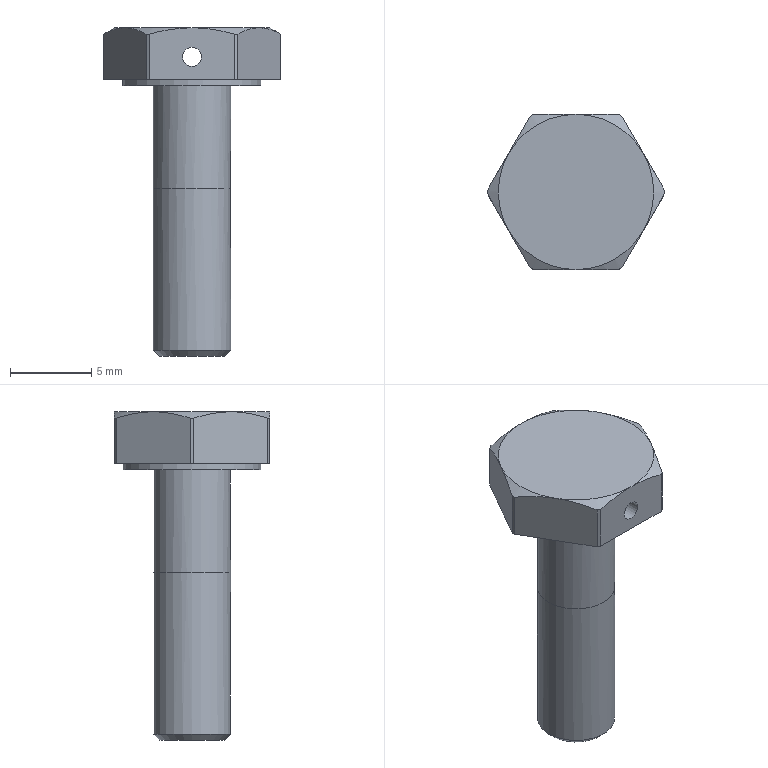Part | NX | features solid 2 | 1 solid | 27 faces | box 10.922 x 9.576 x 20.25 mm | volume 559.779 mm3 | cylinder 10 | plane 10 | cone 7 | commonest cylinder face diameters 10.922 x6 4.763 x2 1.168 x1 8.509 x1
STEP:
#1=CARTESIAN_POINT('',(-2.381,0.,-3.581));
#2=VERTEX_POINT('',#1);
#3=CARTESIAN_POINT('',(0.,0.,-3.581));
#4=DIRECTION('',(0.,0.,-1.));
#5=DIRECTION('',(-1.,0.,0.));
#6=AXIS2_PLACEMENT_3D('',#3,#4,#5);
#7=CIRCLE('',#6,2.381);
#8=EDGE_CURVE('',#2,#2,#7,.T.);
#9=ORIENTED_EDGE('',*,*,#8,.T.);
#10=EDGE_LOOP('',(#9));
#11=FACE_BOUND('',#10,.T.);
#12=CARTESIAN_POINT('',(-2.381,0.,-9.931));
#13=VERTEX_POINT('',#12);
#14=CARTESIAN_POINT('',(-1.866,1.866,-9.931));
#15=CARTESIAN_POINT('',(-2.639,0.,-9.931));
#16=CARTESIAN_POINT('',(-1.866,-1.866,-9.931));
#17=CARTESIAN_POINT('',(0.,-2.639,-9.931));
#18=CARTESIAN_POINT('',(1.866,-1.866,-9.931));
#19=CARTESIAN_POINT('',(2.639,0.,-9.931));
#20=CARTESIAN_POINT('',(1.866,1.866,-9.931));
#21=CARTESIAN_POINT('',(0.,2.639,-9.931));
#22=CARTESIAN_POINT('',(-1.866,1.866,-9.931));
#23=CARTESIAN_POINT('',(-2.639,0.,-9.931));
#24=CARTESIAN_POINT('',(-1.866,-1.866,-9.931));
#25=B_SPLINE_CURVE_WITH_KNOTS('',3,(#14,#15,#16,#17,#18,#19,#20,#21,#22,#23,#24),.UNSPECIFIED.,.T.,.F.,(1,1,1,1,1,1,1,1,1,1,1,1,1,1,1),(-0.375,-0.25,-0.125,0.,0.125,0.25,0.375,0.5,0.625,0.75,0.875,1.,1.125,1.25,1.375),.UNSPECIFIED.);
#26=EDGE_CURVE('',#13,#13,#25,.T.);
#27=ORIENTED_EDGE('',*,*,#26,.T.);
#28=EDGE_LOOP('',(#27));
#29=FACE_BOUND('',#28,.T.);
#30=CARTESIAN_POINT('',(0.,0.,0.));
#31=DIRECTION('',(0.,0.,-1.));
#32=DIRECTION('',(-1.,0.,0.));
#33=AXIS2_PLACEMENT_3D('',#30,#31,#32);
#34=CYLINDRICAL_SURFACE('',#33,2.381);
#35=ADVANCED_FACE('',(#11,#29),#34,.T.);
#36=CARTESIAN_POINT('',(2.627,4.788,-3.175));
#37=VERTEX_POINT('',#36);
#38=CARTESIAN_POINT('',(2.833,4.669,-3.175));
#39=VERTEX_POINT('',#38);
#40=CARTESIAN_POINT('',(0.,0.,-3.175));
#41=DIRECTION('',(0.,0.,-1.));
#42=DIRECTION('',(-1.,0.,0.));
#43=AXIS2_PLACEMENT_3D('',#40,#41,#42);
#44=CIRCLE('',#43,5.461);
#45=EDGE_CURVE('',#37,#39,#44,.T.);
#46=ORIENTED_EDGE('',*,*,#45,.F.);
#47=CARTESIAN_POINT('',(2.627,4.788,-0.3886));
#48=VERTEX_POINT('',#47);
#49=CARTESIAN_POINT('',(2.627,4.788,0.));
#50=DIRECTION('',(0.,0.,-1.));
#51=VECTOR('',#50,1000.);
#52=LINE('',#49,#51);
#53=EDGE_CURVE('',#37,#48,#52,.F.);
#54=ORIENTED_EDGE('',*,*,#53,.T.);
#55=CARTESIAN_POINT('',(2.833,4.669,-0.3886));
#56=VERTEX_POINT('',#55);
#57=CARTESIAN_POINT('',(0.,0.,-0.3886));
#58=DIRECTION('',(0.,0.,-1.));
#59=DIRECTION('',(-1.,0.,0.));
#60=AXIS2_PLACEMENT_3D('',#57,#58,#59);
#61=CIRCLE('',#60,5.461);
#62=EDGE_CURVE('',#48,#56,#61,.T.);
#63=ORIENTED_EDGE('',*,*,#62,.T.);
#64=CARTESIAN_POINT('',(2.833,4.669,0.));
#65=DIRECTION('',(0.,0.,-1.));
#66=VECTOR('',#65,1000.);
#67=LINE('',#64,#66);
#68=EDGE_CURVE('',#56,#39,#67,.T.);
#69=ORIENTED_EDGE('',*,*,#68,.T.);
#70=EDGE_LOOP('',(#46,#54,#63,#69));
#71=FACE_BOUND('',#70,.T.);
#72=CARTESIAN_POINT('',(0.,0.,0.));
#73=DIRECTION('',(0.,0.,-1.));
#74=DIRECTION('',(-1.,0.,0.));
#75=AXIS2_PLACEMENT_3D('',#72,#73,#74);
#76=CYLINDRICAL_SURFACE('',#75,5.461);
#77=ADVANCED_FACE('',(#71),#76,.T.);
#78=CARTESIAN_POINT('',(-2.833,4.669,-0.3886));
#79=VERTEX_POINT('',#78);
#80=CARTESIAN_POINT('',(-2.627,4.788,-0.3886));
#81=VERTEX_POINT('',#80);
#82=CARTESIAN_POINT('',(0.,0.,-0.3886));
#83=DIRECTION('',(0.,0.,-1.));
#84=DIRECTION('',(-1.,0.,0.));
#85=AXIS2_PLACEMENT_3D('',#82,#83,#84);
#86=CIRCLE('',#85,5.461);
#87=EDGE_CURVE('',#79,#81,#86,.T.);
#88=ORIENTED_EDGE('',*,*,#87,.T.);
#89=CARTESIAN_POINT('',(-2.627,4.788,-3.175));
#90=VERTEX_POINT('',#89);
#91=CARTESIAN_POINT('',(-2.627,4.788,0.));
#92=DIRECTION('',(0.,0.,-1.));
#93=VECTOR('',#92,1000.);
#94=LINE('',#91,#93);
#95=EDGE_CURVE('',#81,#90,#94,.T.);
#96=ORIENTED_EDGE('',*,*,#95,.T.);
#97=CARTESIAN_POINT('',(-2.833,4.669,-3.175));
#98=VERTEX_POINT('',#97);
#99=CARTESIAN_POINT('',(0.,0.,-3.175));
#100=DIRECTION('',(0.,0.,-1.));
#101=DIRECTION('',(-1.,0.,0.));
#102=AXIS2_PLACEMENT_3D('',#99,#100,#101);
#103=CIRCLE('',#102,5.461);
#104=EDGE_CURVE('',#98,#90,#103,.T.);
#105=ORIENTED_EDGE('',*,*,#104,.F.);
#106=CARTESIAN_POINT('',(-2.833,4.669,0.));
#107=DIRECTION('',(0.,0.,-1.));
#108=VECTOR('',#107,1000.);
#109=LINE('',#106,#108);
#110=EDGE_CURVE('',#98,#79,#109,.F.);
#111=ORIENTED_EDGE('',*,*,#110,.T.);
#112=EDGE_LOOP('',(#88,#96,#105,#111));
#113=FACE_BOUND('',#112,.T.);
#114=CARTESIAN_POINT('',(0.,0.,0.));
#115=DIRECTION('',(0.,0.,-1.));
#116=DIRECTION('',(-1.,0.,0.));
#117=AXIS2_PLACEMENT_3D('',#114,#115,#116);
#118=CYLINDRICAL_SURFACE('',#117,5.461);
#119=ADVANCED_FACE('',(#113),#118,.T.);
#120=CARTESIAN_POINT('',(-5.46,-0.1193,-0.3886));
#121=VERTEX_POINT('',#120);
#122=CARTESIAN_POINT('',(-5.46,0.1193,-0.3886));
#123=VERTEX_POINT('',#122);
#124=CARTESIAN_POINT('',(0.,0.,-0.3886));
#125=DIRECTION('',(0.,0.,-1.));
#126=DIRECTION('',(-1.,0.,0.));
#127=AXIS2_PLACEMENT_3D('',#124,#125,#126);
#128=CIRCLE('',#127,5.461);
#129=EDGE_CURVE('',#121,#123,#128,.T.);
#130=ORIENTED_EDGE('',*,*,#129,.T.);
#131=CARTESIAN_POINT('',(-5.46,0.1193,-3.175));
#132=VERTEX_POINT('',#131);
#133=CARTESIAN_POINT('',(-5.46,0.1193,0.));
#134=DIRECTION('',(0.,0.,-1.));
#135=VECTOR('',#134,1000.);
#136=LINE('',#133,#135);
#137=EDGE_CURVE('',#123,#132,#136,.T.);
#138=ORIENTED_EDGE('',*,*,#137,.T.);
#139=CARTESIAN_POINT('',(-5.46,-0.1193,-3.175));
#140=VERTEX_POINT('',#139);
#141=CARTESIAN_POINT('',(0.,0.,-3.175));
#142=DIRECTION('',(0.,0.,-1.));
#143=DIRECTION('',(-1.,0.,0.));
#144=AXIS2_PLACEMENT_3D('',#141,#142,#143);
#145=CIRCLE('',#144,5.461);
#146=EDGE_CURVE('',#140,#132,#145,.T.);
#147=ORIENTED_EDGE('',*,*,#146,.F.);
#148=CARTESIAN_POINT('',(-5.46,-0.1193,0.));
#149=DIRECTION('',(0.,0.,-1.));
#150=VECTOR('',#149,1000.);
#151=LINE('',#148,#150);
#152=EDGE_CURVE('',#140,#121,#151,.F.);
#153=ORIENTED_EDGE('',*,*,#152,.T.);
#154=EDGE_LOOP('',(#130,#138,#147,#153));
#155=FACE_BOUND('',#154,.T.);
#156=CARTESIAN_POINT('',(0.,0.,0.));
#157=DIRECTION('',(0.,0.,-1.));
#158=DIRECTION('',(-1.,0.,0.));
#159=AXIS2_PLACEMENT_3D('',#156,#157,#158);
#160=CYLINDRICAL_SURFACE('',#159,5.461);
#161=ADVANCED_FACE('',(#155),#160,.T.);
#162=CARTESIAN_POINT('',(-2.627,-4.788,-0.3886));
#163=VERTEX_POINT('',#162);
#164=CARTESIAN_POINT('',(-2.833,-4.669,-0.3886));
#165=VERTEX_POINT('',#164);
#166=CARTESIAN_POINT('',(0.,0.,-0.3886));
#167=DIRECTION('',(0.,0.,-1.));
#168=DIRECTION('',(-1.,0.,0.));
#169=AXIS2_PLACEMENT_3D('',#166,#167,#168);
#170=CIRCLE('',#169,5.461);
#171=EDGE_CURVE('',#163,#165,#170,.T.);
#172=ORIENTED_EDGE('',*,*,#171,.T.);
#173=CARTESIAN_POINT('',(-2.833,-4.669,-3.175));
#174=VERTEX_POINT('',#173);
#175=CARTESIAN_POINT('',(-2.833,-4.669,0.));
#176=DIRECTION('',(0.,0.,-1.));
#177=VECTOR('',#176,1000.);
#178=LINE('',#175,#177);
#179=EDGE_CURVE('',#165,#174,#178,.T.);
#180=ORIENTED_EDGE('',*,*,#179,.T.);
#181=CARTESIAN_POINT('',(-2.627,-4.788,-3.175));
#182=VERTEX_POINT('',#181);
#183=CARTESIAN_POINT('',(0.,0.,-3.175));
#184=DIRECTION('',(0.,0.,-1.));
#185=DIRECTION('',(-1.,0.,0.));
#186=AXIS2_PLACEMENT_3D('',#183,#184,#185);
#187=CIRCLE('',#186,5.461);
#188=EDGE_CURVE('',#182,#174,#187,.T.);
#189=ORIENTED_EDGE('',*,*,#188,.F.);
#190=CARTESIAN_POINT('',(-2.627,-4.788,0.));
#191=DIRECTION('',(0.,0.,-1.));
#192=VECTOR('',#191,1000.);
#193=LINE('',#190,#192);
#194=EDGE_CURVE('',#182,#163,#193,.F.);
#195=ORIENTED_EDGE('',*,*,#194,.T.);
#196=EDGE_LOOP('',(#172,#180,#189,#195));
#197=FACE_BOUND('',#196,.T.);
#198=CARTESIAN_POINT('',(0.,0.,0.));
#199=DIRECTION('',(0.,0.,-1.));
#200=DIRECTION('',(-1.,0.,0.));
#201=AXIS2_PLACEMENT_3D('',#198,#199,#200);
#202=CYLINDRICAL_SURFACE('',#201,5.461);
#203=ADVANCED_FACE('',(#197),#202,.T.);
#204=CARTESIAN_POINT('',(2.833,-4.669,-0.3886));
#205=VERTEX_POINT('',#204);
#206=CARTESIAN_POINT('',(2.627,-4.788,-0.3886));
#207=VERTEX_POINT('',#206);
#208=CARTESIAN_POINT('',(0.,0.,-0.3886));
#209=DIRECTION('',(0.,0.,-1.));
#210=DIRECTION('',(-1.,0.,0.));
#211=AXIS2_PLACEMENT_3D('',#208,#209,#210);
#212=CIRCLE('',#211,5.461);
#213=EDGE_CURVE('',#205,#207,#212,.T.);
#214=ORIENTED_EDGE('',*,*,#213,.T.);
#215=CARTESIAN_POINT('',(2.627,-4.788,-3.175));
#216=VERTEX_POINT('',#215);
#217=CARTESIAN_POINT('',(2.627,-4.788,0.));
#218=DIRECTION('',(0.,0.,-1.));
#219=VECTOR('',#218,1000.);
#220=LINE('',#217,#219);
#221=EDGE_CURVE('',#207,#216,#220,.T.);
#222=ORIENTED_EDGE('',*,*,#221,.T.);
#223=CARTESIAN_POINT('',(2.833,-4.669,-3.175));
#224=VERTEX_POINT('',#223);
#225=CARTESIAN_POINT('',(0.,0.,-3.175));
#226=DIRECTION('',(0.,0.,-1.));
#227=DIRECTION('',(-1.,0.,0.));
#228=AXIS2_PLACEMENT_3D('',#225,#226,#227);
#229=CIRCLE('',#228,5.461);
#230=EDGE_CURVE('',#224,#216,#229,.T.);
#231=ORIENTED_EDGE('',*,*,#230,.F.);
#232=CARTESIAN_POINT('',(2.833,-4.669,0.));
#233=DIRECTION('',(0.,0.,-1.));
#234=VECTOR('',#233,1000.);
#235=LINE('',#232,#234);
#236=EDGE_CURVE('',#224,#205,#235,.F.);
#237=ORIENTED_EDGE('',*,*,#236,.T.);
#238=EDGE_LOOP('',(#214,#222,#231,#237));
#239=FACE_BOUND('',#238,.T.);
#240=CARTESIAN_POINT('',(0.,0.,0.));
#241=DIRECTION('',(0.,0.,-1.));
#242=DIRECTION('',(-1.,0.,0.));
#243=AXIS2_PLACEMENT_3D('',#240,#241,#242);
#244=CYLINDRICAL_SURFACE('',#243,5.461);
#245=ADVANCED_FACE('',(#239),#244,.T.);
#246=ORIENTED_EDGE('',*,*,#62,.F.);
#247=CARTESIAN_POINT('',(0.,4.788,0.));
#248=VERTEX_POINT('',#247);
#249=CARTESIAN_POINT('',(0.,4.788,0.));
#250=CARTESIAN_POINT('',(0.8868,4.788,0.));
#251=CARTESIAN_POINT('',(1.776,4.788,-0.1525));
#252=CARTESIAN_POINT('',(2.627,4.788,-0.3886));
#253=B_SPLINE_CURVE_WITH_KNOTS('',3,(#249,#250,#251,#252),.UNSPECIFIED.,.F.,.F.,(4,4),(0.007722,0.01038),.UNSPECIFIED.);
#254=EDGE_CURVE('',#48,#248,#253,.F.);
#255=ORIENTED_EDGE('',*,*,#254,.T.);
#256=CARTESIAN_POINT('',(4.146,2.394,0.));
#257=VERTEX_POINT('',#256);
#258=CARTESIAN_POINT('',(0.,0.,0.));
#259=DIRECTION('',(0.,0.,-1.));
#260=DIRECTION('',(-1.,0.,0.));
#261=AXIS2_PLACEMENT_3D('',#258,#259,#260);
#262=CIRCLE('',#261,4.788);
#263=EDGE_CURVE('',#248,#257,#262,.T.);
#264=ORIENTED_EDGE('',*,*,#263,.T.);
#265=CARTESIAN_POINT('',(4.146,2.394,0.));
#266=CARTESIAN_POINT('',(3.703,3.163,0.));
#267=CARTESIAN_POINT('',(3.262,3.925,-0.1503));
#268=CARTESIAN_POINT('',(2.833,4.669,-0.3886));
#269=B_SPLINE_CURVE_WITH_KNOTS('',3,(#265,#266,#267,#268),.UNSPECIFIED.,.F.,.F.,(4,4),(0.002655,0.005296),.UNSPECIFIED.);
#270=EDGE_CURVE('',#257,#56,#269,.T.);
#271=ORIENTED_EDGE('',*,*,#270,.T.);
#272=EDGE_LOOP('',(#246,#255,#264,#271));
#273=FACE_BOUND('',#272,.T.);
#274=CARTESIAN_POINT('',(0.,0.,-0.3886));
#275=DIRECTION('',(0.,0.,-1.));
#276=DIRECTION('',(-1.,0.,0.));
#277=AXIS2_PLACEMENT_3D('',#274,#275,#276);
#278=CONICAL_SURFACE('',#277,5.461,1.047);
#279=ADVANCED_FACE('',(#273),#278,.T.);
#280=CARTESIAN_POINT('',(-4.146,2.394,0.));
#281=VERTEX_POINT('',#280);
#282=CARTESIAN_POINT('',(0.,0.,0.));
#283=DIRECTION('',(0.,0.,-1.));
#284=DIRECTION('',(-1.,0.,0.));
#285=AXIS2_PLACEMENT_3D('',#282,#283,#284);
#286=CIRCLE('',#285,4.788);
#287=EDGE_CURVE('',#281,#248,#286,.T.);
#288=ORIENTED_EDGE('',*,*,#287,.T.);
#289=CARTESIAN_POINT('',(-2.627,4.788,-0.3886));
#290=CARTESIAN_POINT('',(-1.77,4.788,-0.1508));
#291=CARTESIAN_POINT('',(-0.8866,4.788,0.));
#292=CARTESIAN_POINT('',(0.,4.788,0.));
#293=B_SPLINE_CURVE_WITH_KNOTS('',3,(#289,#290,#291,#292),.UNSPECIFIED.,.F.,.F.,(4,4),(0.005068,0.007722),.UNSPECIFIED.);
#294=EDGE_CURVE('',#248,#81,#293,.F.);
#295=ORIENTED_EDGE('',*,*,#294,.T.);
#296=ORIENTED_EDGE('',*,*,#87,.F.);
#297=CARTESIAN_POINT('',(-2.833,4.669,-0.3886));
#298=CARTESIAN_POINT('',(-3.264,3.923,-0.1495));
#299=CARTESIAN_POINT('',(-3.7,3.167,0.));
#300=CARTESIAN_POINT('',(-4.146,2.394,0.));
#301=B_SPLINE_CURVE_WITH_KNOTS('',3,(#297,#298,#299,#300),.UNSPECIFIED.,.F.,.F.,(4,4),(0.00000074,0.002655),.UNSPECIFIED.);
#302=EDGE_CURVE('',#79,#281,#301,.T.);
#303=ORIENTED_EDGE('',*,*,#302,.T.);
#304=EDGE_LOOP('',(#288,#295,#296,#303));
#305=FACE_BOUND('',#304,.T.);
#306=CARTESIAN_POINT('',(0.,0.,-0.3886));
#307=DIRECTION('',(0.,0.,-1.));
#308=DIRECTION('',(-1.,0.,0.));
#309=AXIS2_PLACEMENT_3D('',#306,#307,#308);
#310=CONICAL_SURFACE('',#309,5.461,1.047);
#311=ADVANCED_FACE('',(#305),#310,.T.);
#312=CARTESIAN_POINT('',(-4.146,-2.394,0.));
#313=VERTEX_POINT('',#312);
#314=CARTESIAN_POINT('',(0.,0.,0.));
#315=DIRECTION('',(0.,0.,-1.));
#316=DIRECTION('',(-1.,0.,0.));
#317=AXIS2_PLACEMENT_3D('',#314,#315,#316);
#318=CIRCLE('',#317,4.788);
#319=EDGE_CURVE('',#313,#281,#318,.T.);
#320=ORIENTED_EDGE('',*,*,#319,.T.);
#321=CARTESIAN_POINT('',(-4.146,2.394,0.));
#322=CARTESIAN_POINT('',(-4.59,1.625,0.));
#323=CARTESIAN_POINT('',(-5.031,0.8625,-0.1503));
#324=CARTESIAN_POINT('',(-5.46,0.1193,-0.3886));
#325=B_SPLINE_CURVE_WITH_KNOTS('',3,(#321,#322,#323,#324),.UNSPECIFIED.,.F.,.F.,(4,4),(0.002655,0.005296),.UNSPECIFIED.);
#326=EDGE_CURVE('',#281,#123,#325,.T.);
#327=ORIENTED_EDGE('',*,*,#326,.T.);
#328=ORIENTED_EDGE('',*,*,#129,.F.);
#329=CARTESIAN_POINT('',(-5.46,-0.1193,-0.3886));
#330=CARTESIAN_POINT('',(-5.029,-0.8651,-0.1495));
#331=CARTESIAN_POINT('',(-4.593,-1.621,0.));
#332=CARTESIAN_POINT('',(-4.146,-2.394,0.));
#333=B_SPLINE_CURVE_WITH_KNOTS('',3,(#329,#330,#331,#332),.UNSPECIFIED.,.F.,.F.,(4,4),(0.00000074,0.002655),.UNSPECIFIED.);
#334=EDGE_CURVE('',#121,#313,#333,.T.);
#335=ORIENTED_EDGE('',*,*,#334,.T.);
#336=EDGE_LOOP('',(#320,#327,#328,#335));
#337=FACE_BOUND('',#336,.T.);
#338=CARTESIAN_POINT('',(0.,0.,-0.3886));
#339=DIRECTION('',(0.,0.,-1.));
#340=DIRECTION('',(-1.,0.,0.));
#341=AXIS2_PLACEMENT_3D('',#338,#339,#340);
#342=CONICAL_SURFACE('',#341,5.461,1.047);
#343=ADVANCED_FACE('',(#337),#342,.T.);
#344=CARTESIAN_POINT('',(0.,-4.788,0.));
#345=VERTEX_POINT('',#344);
#346=CARTESIAN_POINT('',(0.,0.,0.));
#347=DIRECTION('',(0.,0.,-1.));
#348=DIRECTION('',(-1.,0.,0.));
#349=AXIS2_PLACEMENT_3D('',#346,#347,#348);
#350=CIRCLE('',#349,4.788);
#351=EDGE_CURVE('',#345,#313,#350,.T.);
#352=ORIENTED_EDGE('',*,*,#351,.T.);
#353=CARTESIAN_POINT('',(-4.146,-2.394,0.));
#354=CARTESIAN_POINT('',(-3.703,-3.163,0.));
#355=CARTESIAN_POINT('',(-3.262,-3.925,-0.1503));
#356=CARTESIAN_POINT('',(-2.833,-4.669,-0.3886));
#357=B_SPLINE_CURVE_WITH_KNOTS('',3,(#353,#354,#355,#356),.UNSPECIFIED.,.F.,.F.,(4,4),(0.002655,0.005296),.UNSPECIFIED.);
#358=EDGE_CURVE('',#313,#165,#357,.T.);
#359=ORIENTED_EDGE('',*,*,#358,.T.);
#360=ORIENTED_EDGE('',*,*,#171,.F.);
#361=CARTESIAN_POINT('',(-2.627,-4.788,-0.3886));
#362=CARTESIAN_POINT('',(-1.77,-4.788,-0.1508));
#363=CARTESIAN_POINT('',(-0.8866,-4.788,0.));
#364=CARTESIAN_POINT('',(0.,-4.788,0.));
#365=B_SPLINE_CURVE_WITH_KNOTS('',3,(#361,#362,#363,#364),.UNSPECIFIED.,.F.,.F.,(4,4),(0.005068,0.007722),.UNSPECIFIED.);
#366=EDGE_CURVE('',#163,#345,#365,.T.);
#367=ORIENTED_EDGE('',*,*,#366,.T.);
#368=EDGE_LOOP('',(#352,#359,#360,#367));
#369=FACE_BOUND('',#368,.T.);
#370=CARTESIAN_POINT('',(0.,0.,-0.3886));
#371=DIRECTION('',(0.,0.,-1.));
#372=DIRECTION('',(-1.,0.,0.));
#373=AXIS2_PLACEMENT_3D('',#370,#371,#372);
#374=CONICAL_SURFACE('',#373,5.461,1.047);
#375=ADVANCED_FACE('',(#369),#374,.T.);
#376=CARTESIAN_POINT('',(4.146,-2.394,0.));
#377=VERTEX_POINT('',#376);
#378=CARTESIAN_POINT('',(0.,0.,0.));
#379=DIRECTION('',(0.,0.,-1.));
#380=DIRECTION('',(-1.,0.,0.));
#381=AXIS2_PLACEMENT_3D('',#378,#379,#380);
#382=CIRCLE('',#381,4.788);
#383=EDGE_CURVE('',#377,#345,#382,.T.);
#384=ORIENTED_EDGE('',*,*,#383,.T.);
#385=CARTESIAN_POINT('',(0.,-4.788,0.));
#386=CARTESIAN_POINT('',(0.8868,-4.788,0.));
#387=CARTESIAN_POINT('',(1.776,-4.788,-0.1525));
#388=CARTESIAN_POINT('',(2.627,-4.788,-0.3886));
#389=B_SPLINE_CURVE_WITH_KNOTS('',3,(#385,#386,#387,#388),.UNSPECIFIED.,.F.,.F.,(4,4),(0.007722,0.01038),.UNSPECIFIED.);
#390=EDGE_CURVE('',#345,#207,#389,.T.);
#391=ORIENTED_EDGE('',*,*,#390,.T.);
#392=ORIENTED_EDGE('',*,*,#213,.F.);
#393=CARTESIAN_POINT('',(2.833,-4.669,-0.3886));
#394=CARTESIAN_POINT('',(3.264,-3.923,-0.1495));
#395=CARTESIAN_POINT('',(3.7,-3.167,0.));
#396=CARTESIAN_POINT('',(4.146,-2.394,0.));
#397=B_SPLINE_CURVE_WITH_KNOTS('',3,(#393,#394,#395,#396),.UNSPECIFIED.,.F.,.F.,(4,4),(0.00000074,0.002655),.UNSPECIFIED.);
#398=EDGE_CURVE('',#205,#377,#397,.T.);
#399=ORIENTED_EDGE('',*,*,#398,.T.);
#400=EDGE_LOOP('',(#384,#391,#392,#399));
#401=FACE_BOUND('',#400,.T.);
#402=CARTESIAN_POINT('',(0.,0.,-0.3886));
#403=DIRECTION('',(0.,0.,-1.));
#404=DIRECTION('',(-1.,0.,0.));
#405=AXIS2_PLACEMENT_3D('',#402,#403,#404);
#406=CONICAL_SURFACE('',#405,5.461,1.047);
#407=ADVANCED_FACE('',(#401),#406,.T.);
#408=ORIENTED_EDGE('',*,*,#104,.T.);
#409=CARTESIAN_POINT('',(4.255,4.788,-3.175));
#410=DIRECTION('',(1.,0.,0.));
#411=VECTOR('',#410,1000.);
#412=LINE('',#409,#411);
#413=EDGE_CURVE('',#90,#37,#412,.T.);
#414=ORIENTED_EDGE('',*,*,#413,.T.);
#415=ORIENTED_EDGE('',*,*,#45,.T.);
#416=CARTESIAN_POINT('',(5.46,0.1193,-3.175));
#417=VERTEX_POINT('',#416);
#418=CARTESIAN_POINT('',(5.21,0.5517,-3.175));
#419=DIRECTION('',(0.5,-0.866,0.));
#420=VECTOR('',#419,1000.);
#421=LINE('',#418,#420);
#422=EDGE_CURVE('',#39,#417,#421,.T.);
#423=ORIENTED_EDGE('',*,*,#422,.T.);
#424=CARTESIAN_POINT('',(5.46,-0.1193,-3.175));
#425=VERTEX_POINT('',#424);
#426=CARTESIAN_POINT('',(0.,0.,-3.175));
#427=DIRECTION('',(0.,0.,-1.));
#428=DIRECTION('',(-1.,0.,0.));
#429=AXIS2_PLACEMENT_3D('',#426,#427,#428);
#430=CIRCLE('',#429,5.461);
#431=EDGE_CURVE('',#417,#425,#430,.T.);
#432=ORIENTED_EDGE('',*,*,#431,.T.);
#433=CARTESIAN_POINT('',(5.21,-0.5517,-3.175));
#434=DIRECTION('',(-0.5,-0.866,0.));
#435=VECTOR('',#434,1000.);
#436=LINE('',#433,#435);
#437=EDGE_CURVE('',#425,#224,#436,.T.);
#438=ORIENTED_EDGE('',*,*,#437,.T.);
#439=ORIENTED_EDGE('',*,*,#230,.T.);
#440=CARTESIAN_POINT('',(4.255,-4.788,-3.175));
#441=DIRECTION('',(-1.,0.,0.));
#442=VECTOR('',#441,1000.);
#443=LINE('',#440,#442);
#444=EDGE_CURVE('',#216,#182,#443,.T.);
#445=ORIENTED_EDGE('',*,*,#444,.T.);
#446=ORIENTED_EDGE('',*,*,#188,.T.);
#447=CARTESIAN_POINT('',(-3.083,-4.236,-3.175));
#448=DIRECTION('',(-0.5,0.866,0.));
#449=VECTOR('',#448,1000.);
#450=LINE('',#447,#449);
#451=EDGE_CURVE('',#174,#140,#450,.T.);
#452=ORIENTED_EDGE('',*,*,#451,.T.);
#453=ORIENTED_EDGE('',*,*,#146,.T.);
#454=CARTESIAN_POINT('',(-3.083,4.236,-3.175));
#455=DIRECTION('',(0.5,0.866,0.));
#456=VECTOR('',#455,1000.);
#457=LINE('',#454,#456);
#458=EDGE_CURVE('',#132,#98,#457,.T.);
#459=ORIENTED_EDGE('',*,*,#458,.T.);
#460=EDGE_LOOP('',(#408,#414,#415,#423,#432,#438,#439,#445,#446,#452,#453,#459));
#461=FACE_BOUND('',#460,.T.);
#462=CARTESIAN_POINT('',(-4.255,0.,-3.175));
#463=VERTEX_POINT('',#462);
#464=CARTESIAN_POINT('',(0.,0.,-3.175));
#465=DIRECTION('',(0.,0.,-1.));
#466=DIRECTION('',(-1.,0.,0.));
#467=AXIS2_PLACEMENT_3D('',#464,#465,#466);
#468=CIRCLE('',#467,4.255);
#469=EDGE_CURVE('',#463,#463,#468,.T.);
#470=ORIENTED_EDGE('',*,*,#469,.F.);
#471=EDGE_LOOP('',(#470));
#472=FACE_BOUND('',#471,.T.);
#473=CARTESIAN_POINT('',(4.255,0.,-3.175));
#474=DIRECTION('',(0.,0.,-1.));
#475=DIRECTION('',(-1.,0.,0.));
#476=AXIS2_PLACEMENT_3D('',#473,#474,#475);
#477=PLANE('',#476);
#478=ADVANCED_FACE('',(#461,#472),#477,.T.);
#479=CARTESIAN_POINT('',(5.46,0.1193,-0.3886));
#480=VERTEX_POINT('',#479);
#481=CARTESIAN_POINT('',(5.46,-0.1193,-0.3886));
#482=VERTEX_POINT('',#481);
#483=CARTESIAN_POINT('',(0.,0.,-0.3886));
#484=DIRECTION('',(0.,0.,-1.));
#485=DIRECTION('',(-1.,0.,0.));
#486=AXIS2_PLACEMENT_3D('',#483,#484,#485);
#487=CIRCLE('',#486,5.461);
#488=EDGE_CURVE('',#480,#482,#487,.T.);
#489=ORIENTED_EDGE('',*,*,#488,.T.);
#490=CARTESIAN_POINT('',(5.46,-0.1193,0.));
#491=DIRECTION('',(0.,0.,-1.));
#492=VECTOR('',#491,1000.);
#493=LINE('',#490,#492);
#494=EDGE_CURVE('',#482,#425,#493,.T.);
#495=ORIENTED_EDGE('',*,*,#494,.T.);
#496=ORIENTED_EDGE('',*,*,#431,.F.);
#497=CARTESIAN_POINT('',(5.46,0.1193,0.));
#498=DIRECTION('',(0.,0.,-1.));
#499=VECTOR('',#498,1000.);
#500=LINE('',#497,#499);
#501=EDGE_CURVE('',#417,#480,#500,.F.);
#502=ORIENTED_EDGE('',*,*,#501,.T.);
#503=EDGE_LOOP('',(#489,#495,#496,#502));
#504=FACE_BOUND('',#503,.T.);
#505=CARTESIAN_POINT('',(0.,0.,0.));
#506=DIRECTION('',(0.,0.,-1.));
#507=DIRECTION('',(-1.,0.,0.));
#508=AXIS2_PLACEMENT_3D('',#505,#506,#507);
#509=CYLINDRICAL_SURFACE('',#508,5.461);
#510=ADVANCED_FACE('',(#504),#509,.T.);
#511=CARTESIAN_POINT('',(0.,0.,0.));
#512=DIRECTION('',(0.,0.,-1.));
#513=DIRECTION('',(-1.,0.,0.));
#514=AXIS2_PLACEMENT_3D('',#511,#512,#513);
#515=CIRCLE('',#514,4.788);
#516=EDGE_CURVE('',#257,#377,#515,.T.);
#517=ORIENTED_EDGE('',*,*,#516,.T.);
#518=CARTESIAN_POINT('',(4.146,-2.394,0.));
#519=CARTESIAN_POINT('',(4.59,-1.625,0.));
#520=CARTESIAN_POINT('',(5.031,-0.8625,-0.1503));
#521=CARTESIAN_POINT('',(5.46,-0.1193,-0.3886));
#522=B_SPLINE_CURVE_WITH_KNOTS('',3,(#518,#519,#520,#521),.UNSPECIFIED.,.F.,.F.,(4,4),(0.002655,0.005296),.UNSPECIFIED.);
#523=EDGE_CURVE('',#377,#482,#522,.T.);
#524=ORIENTED_EDGE('',*,*,#523,.T.);
#525=ORIENTED_EDGE('',*,*,#488,.F.);
#526=CARTESIAN_POINT('',(5.46,0.1193,-0.3886));
#527=CARTESIAN_POINT('',(5.029,0.8651,-0.1495));
#528=CARTESIAN_POINT('',(4.593,1.621,0.));
#529=CARTESIAN_POINT('',(4.146,2.394,0.));
#530=B_SPLINE_CURVE_WITH_KNOTS('',3,(#526,#527,#528,#529),.UNSPECIFIED.,.F.,.F.,(4,4),(0.00000074,0.002655),.UNSPECIFIED.);
#531=EDGE_CURVE('',#480,#257,#530,.T.);
#532=ORIENTED_EDGE('',*,*,#531,.T.);
#533=EDGE_LOOP('',(#517,#524,#525,#532));
#534=FACE_BOUND('',#533,.T.);
#535=CARTESIAN_POINT('',(0.,0.,-0.3886));
#536=DIRECTION('',(0.,0.,-1.));
#537=DIRECTION('',(-1.,0.,0.));
#538=AXIS2_PLACEMENT_3D('',#535,#536,#537);
#539=CONICAL_SURFACE('',#538,5.461,1.047);
#540=ADVANCED_FACE('',(#534),#539,.T.);
#541=ORIENTED_EDGE('',*,*,#287,.F.);
#542=ORIENTED_EDGE('',*,*,#319,.F.);
#543=ORIENTED_EDGE('',*,*,#351,.F.);
#544=ORIENTED_EDGE('',*,*,#383,.F.);
#545=ORIENTED_EDGE('',*,*,#516,.F.);
#546=ORIENTED_EDGE('',*,*,#263,.F.);
#547=EDGE_LOOP('',(#541,#542,#543,#544,#545,#546));
#548=FACE_BOUND('',#547,.T.);
#549=CARTESIAN_POINT('',(4.788,0.,0.));
#550=DIRECTION('',(0.,0.,1.));
#551=DIRECTION('',(1.,0.,0.));
#552=AXIS2_PLACEMENT_3D('',#549,#550,#551);
#553=PLANE('',#552);
#554=ADVANCED_FACE('',(#548),#553,.T.);
#555=CARTESIAN_POINT('',(-2.,0.,-20.25));
#556=VERTEX_POINT('',#555);
#557=CARTESIAN_POINT('',(0.,0.,-20.25));
#558=DIRECTION('',(0.,0.,-1.));
#559=DIRECTION('',(-1.,0.,0.));
#560=AXIS2_PLACEMENT_3D('',#557,#558,#559);
#561=CIRCLE('',#560,2.);
#562=EDGE_CURVE('',#556,#556,#561,.T.);
#563=ORIENTED_EDGE('',*,*,#562,.T.);
#564=EDGE_LOOP('',(#563));
#565=FACE_BOUND('',#564,.T.);
#566=CARTESIAN_POINT('',(0.,0.,-20.25));
#567=DIRECTION('',(0.,0.,-1.));
#568=DIRECTION('',(-1.,0.,0.));
#569=AXIS2_PLACEMENT_3D('',#566,#567,#568);
#570=PLANE('',#569);
#571=ADVANCED_FACE('',(#565),#570,.T.);
#572=CARTESIAN_POINT('',(-2.381,0.,-19.869));
#573=VERTEX_POINT('',#572);
#574=CARTESIAN_POINT('',(0.,0.,-19.869));
#575=DIRECTION('',(0.,0.,-1.));
#576=DIRECTION('',(-1.,0.,0.));
#577=AXIS2_PLACEMENT_3D('',#574,#575,#576);
#578=CIRCLE('',#577,2.381);
#579=EDGE_CURVE('',#573,#573,#578,.T.);
#580=ORIENTED_EDGE('',*,*,#579,.T.);
#581=EDGE_LOOP('',(#580));
#582=FACE_BOUND('',#581,.T.);
#583=ORIENTED_EDGE('',*,*,#562,.F.);
#584=EDGE_LOOP('',(#583));
#585=FACE_BOUND('',#584,.T.);
#586=CARTESIAN_POINT('',(0.,0.,-20.25));
#587=DIRECTION('',(0.,0.,1.));
#588=DIRECTION('',(1.,0.,0.));
#589=AXIS2_PLACEMENT_3D('',#586,#587,#588);
#590=CONICAL_SURFACE('',#589,2.,0.7854);
#591=ADVANCED_FACE('',(#582,#585),#590,.T.);
#592=ORIENTED_EDGE('',*,*,#26,.F.);
#593=EDGE_LOOP('',(#592));
#594=FACE_BOUND('',#593,.T.);
#595=ORIENTED_EDGE('',*,*,#579,.F.);
#596=EDGE_LOOP('',(#595));
#597=FACE_BOUND('',#596,.T.);
#598=CARTESIAN_POINT('',(0.,0.,0.));
#599=DIRECTION('',(0.,0.,-1.));
#600=DIRECTION('',(-1.,0.,0.));
#601=AXIS2_PLACEMENT_3D('',#598,#599,#600);
#602=CYLINDRICAL_SURFACE('',#601,2.381);
#603=ADVANCED_FACE('',(#594,#597),#602,.T.);
#604=CARTESIAN_POINT('',(-4.255,0.,-3.581));
#605=VERTEX_POINT('',#604);
#606=CARTESIAN_POINT('',(0.,0.,-3.581));
#607=DIRECTION('',(0.,0.,-1.));
#608=DIRECTION('',(-1.,0.,0.));
#609=AXIS2_PLACEMENT_3D('',#606,#607,#608);
#610=CIRCLE('',#609,4.255);
#611=EDGE_CURVE('',#605,#605,#610,.T.);
#612=ORIENTED_EDGE('',*,*,#611,.T.);
#613=EDGE_LOOP('',(#612));
#614=FACE_BOUND('',#613,.T.);
#615=ORIENTED_EDGE('',*,*,#8,.F.);
#616=EDGE_LOOP('',(#615));
#617=FACE_BOUND('',#616,.T.);
#618=CARTESIAN_POINT('',(2.381,0.,-3.581));
#619=DIRECTION('',(0.,0.,-1.));
#620=DIRECTION('',(-1.,0.,0.));
#621=AXIS2_PLACEMENT_3D('',#618,#619,#620);
#622=PLANE('',#621);
#623=ADVANCED_FACE('',(#614,#617),#622,.T.);
#624=ORIENTED_EDGE('',*,*,#469,.T.);
#625=EDGE_LOOP('',(#624));
#626=FACE_BOUND('',#625,.T.);
#627=ORIENTED_EDGE('',*,*,#611,.F.);
#628=EDGE_LOOP('',(#627));
#629=FACE_BOUND('',#628,.T.);
#630=CARTESIAN_POINT('',(0.,0.,0.));
#631=DIRECTION('',(0.,0.,-1.));
#632=DIRECTION('',(-1.,0.,0.));
#633=AXIS2_PLACEMENT_3D('',#630,#631,#632);
#634=CYLINDRICAL_SURFACE('',#633,4.255);
#635=ADVANCED_FACE('',(#626,#629),#634,.T.);
#636=ORIENTED_EDGE('',*,*,#422,.F.);
#637=ORIENTED_EDGE('',*,*,#68,.F.);
#638=ORIENTED_EDGE('',*,*,#270,.F.);
#639=ORIENTED_EDGE('',*,*,#531,.F.);
#640=ORIENTED_EDGE('',*,*,#501,.F.);
#641=EDGE_LOOP('',(#636,#637,#638,#639,#640));
#642=FACE_BOUND('',#641,.T.);
#643=CARTESIAN_POINT('',(5.529,0.,-22.275));
#644=DIRECTION('',(0.866,0.5,0.));
#645=DIRECTION('',(-0.5,0.866,0.));
#646=AXIS2_PLACEMENT_3D('',#643,#644,#645);
#647=PLANE('',#646);
#648=ADVANCED_FACE('',(#642),#647,.T.);
#649=ORIENTED_EDGE('',*,*,#437,.F.);
#650=ORIENTED_EDGE('',*,*,#494,.F.);
#651=ORIENTED_EDGE('',*,*,#523,.F.);
#652=ORIENTED_EDGE('',*,*,#398,.F.);
#653=ORIENTED_EDGE('',*,*,#236,.F.);
#654=EDGE_LOOP('',(#649,#650,#651,#652,#653));
#655=FACE_BOUND('',#654,.T.);
#656=CARTESIAN_POINT('',(2.764,-4.788,-22.275));
#657=DIRECTION('',(0.866,-0.5,0.));
#658=DIRECTION('',(0.5,0.866,0.));
#659=AXIS2_PLACEMENT_3D('',#656,#657,#658);
#660=PLANE('',#659);
#661=ADVANCED_FACE('',(#655),#660,.T.);
#662=CARTESIAN_POINT('',(0.,-4.788,-2.375));
#663=VERTEX_POINT('',#662);
#664=CARTESIAN_POINT('',(0.,-4.788,-1.791));
#665=DIRECTION('',(0.,-1.,0.));
#666=DIRECTION('',(0.,0.,-1.));
#667=AXIS2_PLACEMENT_3D('',#664,#665,#666);
#668=CIRCLE('',#667,0.5842);
#669=EDGE_CURVE('',#663,#663,#668,.T.);
#670=ORIENTED_EDGE('',*,*,#669,.F.);
#671=EDGE_LOOP('',(#670));
#672=FACE_BOUND('',#671,.T.);
#673=ORIENTED_EDGE('',*,*,#444,.F.);
#674=ORIENTED_EDGE('',*,*,#221,.F.);
#675=ORIENTED_EDGE('',*,*,#390,.F.);
#676=ORIENTED_EDGE('',*,*,#366,.F.);
#677=ORIENTED_EDGE('',*,*,#194,.F.);
#678=EDGE_LOOP('',(#673,#674,#675,#676,#677));
#679=FACE_BOUND('',#678,.T.);
#680=CARTESIAN_POINT('',(-2.764,-4.788,-22.275));
#681=DIRECTION('',(0.,-1.,0.));
#682=DIRECTION('',(0.,0.,-1.));
#683=AXIS2_PLACEMENT_3D('',#680,#681,#682);
#684=PLANE('',#683);
#685=ADVANCED_FACE('',(#672,#679),#684,.T.);
#686=ORIENTED_EDGE('',*,*,#451,.F.);
#687=ORIENTED_EDGE('',*,*,#179,.F.);
#688=ORIENTED_EDGE('',*,*,#358,.F.);
#689=ORIENTED_EDGE('',*,*,#334,.F.);
#690=ORIENTED_EDGE('',*,*,#152,.F.);
#691=EDGE_LOOP('',(#686,#687,#688,#689,#690));
#692=FACE_BOUND('',#691,.T.);
#693=CARTESIAN_POINT('',(-5.529,0.,-22.275));
#694=DIRECTION('',(-0.866,-0.5,0.));
#695=DIRECTION('',(0.5,-0.866,0.));
#696=AXIS2_PLACEMENT_3D('',#693,#694,#695);
#697=PLANE('',#696);
#698=ADVANCED_FACE('',(#692),#697,.T.);
#699=ORIENTED_EDGE('',*,*,#458,.F.);
#700=ORIENTED_EDGE('',*,*,#137,.F.);
#701=ORIENTED_EDGE('',*,*,#326,.F.);
#702=ORIENTED_EDGE('',*,*,#302,.F.);
#703=ORIENTED_EDGE('',*,*,#110,.F.);
#704=EDGE_LOOP('',(#699,#700,#701,#702,#703));
#705=FACE_BOUND('',#704,.T.);
#706=CARTESIAN_POINT('',(-2.764,4.788,-22.275));
#707=DIRECTION('',(-0.866,0.5,0.));
#708=DIRECTION('',(-0.5,-0.866,0.));
#709=AXIS2_PLACEMENT_3D('',#706,#707,#708);
#710=PLANE('',#709);
#711=ADVANCED_FACE('',(#705),#710,.T.);
#712=CARTESIAN_POINT('',(0.,4.788,-1.206));
#713=VERTEX_POINT('',#712);
#714=CARTESIAN_POINT('',(0.,4.788,-1.791));
#715=DIRECTION('',(0.,1.,0.));
#716=DIRECTION('',(0.,0.,1.));
#717=AXIS2_PLACEMENT_3D('',#714,#715,#716);
#718=CIRCLE('',#717,0.5842);
#719=EDGE_CURVE('',#713,#713,#718,.T.);
#720=ORIENTED_EDGE('',*,*,#719,.F.);
#721=EDGE_LOOP('',(#720));
#722=FACE_BOUND('',#721,.T.);
#723=ORIENTED_EDGE('',*,*,#413,.F.);
#724=ORIENTED_EDGE('',*,*,#95,.F.);
#725=ORIENTED_EDGE('',*,*,#294,.F.);
#726=ORIENTED_EDGE('',*,*,#254,.F.);
#727=ORIENTED_EDGE('',*,*,#53,.F.);
#728=EDGE_LOOP('',(#723,#724,#725,#726,#727));
#729=FACE_BOUND('',#728,.T.);
#730=CARTESIAN_POINT('',(2.764,4.788,-22.275));
#731=DIRECTION('',(0.,1.,0.));
#732=DIRECTION('',(0.,0.,1.));
#733=AXIS2_PLACEMENT_3D('',#730,#731,#732);
#734=PLANE('',#733);
#735=ADVANCED_FACE('',(#722,#729),#734,.T.);
#736=ORIENTED_EDGE('',*,*,#669,.T.);
#737=EDGE_LOOP('',(#736));
#738=FACE_BOUND('',#737,.T.);
#739=ORIENTED_EDGE('',*,*,#719,.T.);
#740=EDGE_LOOP('',(#739));
#741=FACE_BOUND('',#740,.T.);
#742=CARTESIAN_POINT('',(0.,5.267,-1.791));
#743=DIRECTION('',(0.,-1.,0.));
#744=DIRECTION('',(0.,0.,-1.));
#745=AXIS2_PLACEMENT_3D('',#742,#743,#744);
#746=CYLINDRICAL_SURFACE('',#745,0.5842);
#747=ADVANCED_FACE('',(#738,#741),#746,.F.);
#748=CLOSED_SHELL('',(#35,#77,#119,#161,#203,#245,#279,#311,#343,#375,#407,#478,#510,#540,#554,#571,#591,#603,#623,#635,#648,#661,#685,#698,#711,#735,#747));
#749=MANIFOLD_SOLID_BREP('',#748);
#750=(LENGTH_UNIT()NAMED_UNIT(*)SI_UNIT(.MILLI.,.METRE.));
#751=UNCERTAINTY_MEASURE_WITH_UNIT(LENGTH_MEASURE(0.0508),#750,'','');
#752=(NAMED_UNIT(*)PLANE_ANGLE_UNIT()SI_UNIT($,.RADIAN.));
#753=(NAMED_UNIT(*)SI_UNIT($,.STERADIAN.)SOLID_ANGLE_UNIT());
#754=(GEOMETRIC_REPRESENTATION_CONTEXT(3)GLOBAL_UNCERTAINTY_ASSIGNED_CONTEXT((#751))GLOBAL_UNIT_ASSIGNED_CONTEXT((#750,#752,#753))REPRESENTATION_CONTEXT('',''));
#755=ADVANCED_BREP_SHAPE_REPRESENTATION('',(#749),#754);